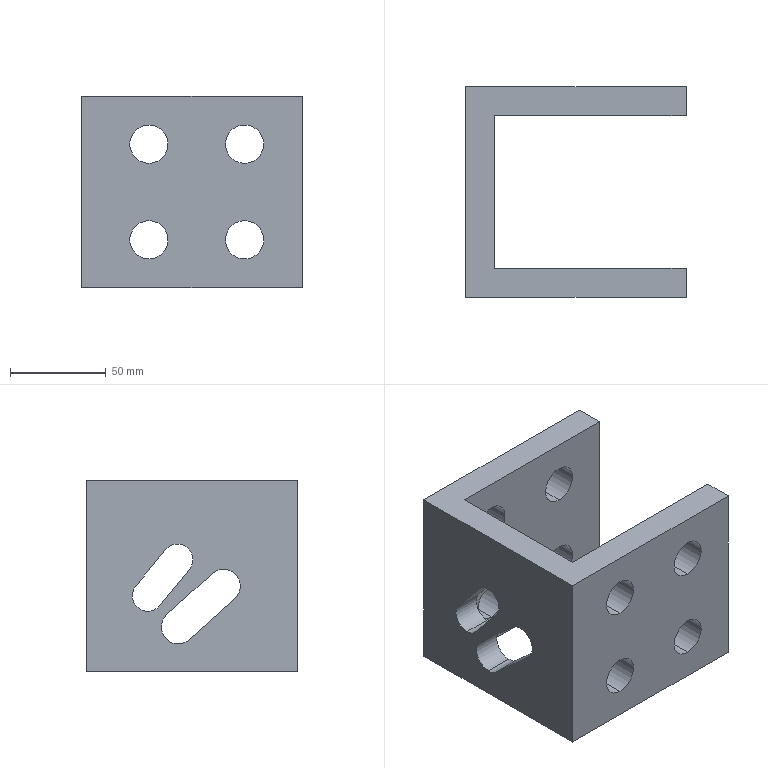Part | SolidWorks | features ICE 2, Extrusion 1 | 1 solid | 36 faces | box 115 x 110 x 100 mm | volume 406186 mm3 | cylinder 22 | plane 14 | commonest cylinder face diameters 20 x16 16.141 x3 17.644 x3
STEP:
#1=CARTESIAN_POINT('',(-15.,47.219,14.48));
#2=VERTEX_POINT('',#1);
#3=CARTESIAN_POINT('',(-15.,53.133,29.848));
#4=VERTEX_POINT('',#3);
#5=CARTESIAN_POINT('',(-15.,47.219,23.302));
#6=DIRECTION('',(1.,0.,0.));
#7=DIRECTION('',(0.,0.,-1.));
#8=AXIS2_PLACEMENT_3D('',#5,#6,#7);
#9=CIRCLE('',#8,8.822);
#10=EDGE_CURVE('',#2,#4,#9,.T.);
#11=ORIENTED_EDGE('',*,*,#10,.F.);
#12=CARTESIAN_POINT('',(0.,47.219,14.48));
#13=VERTEX_POINT('',#12);
#14=CARTESIAN_POINT('',(-500.,47.219,14.48));
#15=DIRECTION('',(1.,0.,0.));
#16=VECTOR('',#15,1000.);
#17=LINE('',#14,#16);
#18=EDGE_CURVE('',#2,#13,#17,.T.);
#19=ORIENTED_EDGE('',*,*,#18,.T.);
#20=CARTESIAN_POINT('',(0.,53.133,29.848));
#21=VERTEX_POINT('',#20);
#22=CARTESIAN_POINT('',(0.,47.219,23.302));
#23=DIRECTION('',(1.,0.,0.));
#24=DIRECTION('',(0.,0.,-1.));
#25=AXIS2_PLACEMENT_3D('',#22,#23,#24);
#26=CIRCLE('',#25,8.822);
#27=EDGE_CURVE('',#13,#21,#26,.T.);
#28=ORIENTED_EDGE('',*,*,#27,.T.);
#29=CARTESIAN_POINT('',(-500.,53.133,29.848));
#30=DIRECTION('',(1.,0.,0.));
#31=VECTOR('',#30,1000.);
#32=LINE('',#29,#31);
#33=EDGE_CURVE('',#4,#21,#32,.T.);
#34=ORIENTED_EDGE('',*,*,#33,.F.);
#35=EDGE_LOOP('',(#11,#19,#28,#34));
#36=FACE_OUTER_BOUND('',#35,.T.);
#37=CARTESIAN_POINT('',(-500.,47.219,23.302));
#38=DIRECTION('',(1.,0.,0.));
#39=DIRECTION('',(0.,0.,-1.));
#40=AXIS2_PLACEMENT_3D('',#37,#38,#39);
#41=CYLINDRICAL_SURFACE('',#40,8.822);
#42=ADVANCED_FACE('',(#36),#41,.F.);
#43=CARTESIAN_POINT('',(-15.,63.133,31.531));
#44=VERTEX_POINT('',#43);
#45=CARTESIAN_POINT('',(-15.,69.375,44.718));
#46=VERTEX_POINT('',#45);
#47=CARTESIAN_POINT('',(-15.,63.133,39.601));
#48=DIRECTION('',(1.,0.,0.));
#49=DIRECTION('',(0.,0.,-1.));
#50=AXIS2_PLACEMENT_3D('',#47,#48,#49);
#51=CIRCLE('',#50,8.071);
#52=EDGE_CURVE('',#44,#46,#51,.T.);
#53=ORIENTED_EDGE('',*,*,#52,.F.);
#54=CARTESIAN_POINT('',(0.,63.133,31.531));
#55=VERTEX_POINT('',#54);
#56=CARTESIAN_POINT('',(-500.,63.133,31.531));
#57=DIRECTION('',(1.,0.,0.));
#58=VECTOR('',#57,1000.);
#59=LINE('',#56,#58);
#60=EDGE_CURVE('',#44,#55,#59,.T.);
#61=ORIENTED_EDGE('',*,*,#60,.T.);
#62=CARTESIAN_POINT('',(0.,69.375,44.718));
#63=VERTEX_POINT('',#62);
#64=CARTESIAN_POINT('',(0.,63.133,39.601));
#65=DIRECTION('',(1.,0.,0.));
#66=DIRECTION('',(0.,0.,-1.));
#67=AXIS2_PLACEMENT_3D('',#64,#65,#66);
#68=CIRCLE('',#67,8.071);
#69=EDGE_CURVE('',#55,#63,#68,.T.);
#70=ORIENTED_EDGE('',*,*,#69,.T.);
#71=CARTESIAN_POINT('',(-500.,69.375,44.718));
#72=DIRECTION('',(1.,0.,0.));
#73=VECTOR('',#72,1000.);
#74=LINE('',#71,#73);
#75=EDGE_CURVE('',#46,#63,#74,.T.);
#76=ORIENTED_EDGE('',*,*,#75,.F.);
#77=EDGE_LOOP('',(#53,#61,#70,#76));
#78=FACE_OUTER_BOUND('',#77,.T.);
#79=CARTESIAN_POINT('',(-500.,63.133,39.601));
#80=DIRECTION('',(1.,0.,0.));
#81=DIRECTION('',(0.,0.,-1.));
#82=AXIS2_PLACEMENT_3D('',#79,#80,#81);
#83=CYLINDRICAL_SURFACE('',#82,8.071);
#84=ADVANCED_FACE('',(#78),#83,.F.);
#85=CARTESIAN_POINT('',(70.,80.,15.));
#86=VERTEX_POINT('',#85);
#87=CARTESIAN_POINT('',(70.,80.,35.));
#88=VERTEX_POINT('',#87);
#89=CARTESIAN_POINT('',(70.,80.,25.));
#90=DIRECTION('',(0.,1.,0.));
#91=DIRECTION('',(0.,0.,1.));
#92=AXIS2_PLACEMENT_3D('',#89,#90,#91);
#93=CIRCLE('',#92,10.);
#94=EDGE_CURVE('',#86,#88,#93,.T.);
#95=ORIENTED_EDGE('',*,*,#94,.F.);
#96=CARTESIAN_POINT('',(70.,95.,15.));
#97=VERTEX_POINT('',#96);
#98=CARTESIAN_POINT('',(70.,-405.,15.));
#99=DIRECTION('',(0.,1.,0.));
#100=VECTOR('',#99,1000.);
#101=LINE('',#98,#100);
#102=EDGE_CURVE('',#86,#97,#101,.T.);
#103=ORIENTED_EDGE('',*,*,#102,.T.);
#104=CARTESIAN_POINT('',(70.,95.,35.));
#105=VERTEX_POINT('',#104);
#106=CARTESIAN_POINT('',(70.,95.,25.));
#107=DIRECTION('',(0.,1.,0.));
#108=DIRECTION('',(0.,0.,1.));
#109=AXIS2_PLACEMENT_3D('',#106,#107,#108);
#110=CIRCLE('',#109,10.);
#111=EDGE_CURVE('',#97,#105,#110,.T.);
#112=ORIENTED_EDGE('',*,*,#111,.T.);
#113=CARTESIAN_POINT('',(70.,-405.,35.));
#114=DIRECTION('',(0.,1.,0.));
#115=VECTOR('',#114,1000.);
#116=LINE('',#113,#115);
#117=EDGE_CURVE('',#88,#105,#116,.T.);
#118=ORIENTED_EDGE('',*,*,#117,.F.);
#119=EDGE_LOOP('',(#95,#103,#112,#118));
#120=FACE_OUTER_BOUND('',#119,.T.);
#121=CARTESIAN_POINT('',(70.,-405.,25.));
#122=DIRECTION('',(0.,1.,0.));
#123=DIRECTION('',(0.,0.,1.));
#124=AXIS2_PLACEMENT_3D('',#121,#122,#123);
#125=CYLINDRICAL_SURFACE('',#124,10.);
#126=ADVANCED_FACE('',(#120),#125,.F.);
#127=CARTESIAN_POINT('',(20.,80.,65.));
#128=VERTEX_POINT('',#127);
#129=CARTESIAN_POINT('',(20.,80.,85.));
#130=VERTEX_POINT('',#129);
#131=CARTESIAN_POINT('',(20.,80.,75.));
#132=DIRECTION('',(0.,1.,0.));
#133=DIRECTION('',(0.,0.,1.));
#134=AXIS2_PLACEMENT_3D('',#131,#132,#133);
#135=CIRCLE('',#134,10.);
#136=EDGE_CURVE('',#128,#130,#135,.T.);
#137=ORIENTED_EDGE('',*,*,#136,.F.);
#138=CARTESIAN_POINT('',(20.,95.,65.));
#139=VERTEX_POINT('',#138);
#140=CARTESIAN_POINT('',(20.,-405.,65.));
#141=DIRECTION('',(0.,1.,0.));
#142=VECTOR('',#141,1000.);
#143=LINE('',#140,#142);
#144=EDGE_CURVE('',#128,#139,#143,.T.);
#145=ORIENTED_EDGE('',*,*,#144,.T.);
#146=CARTESIAN_POINT('',(20.,95.,85.));
#147=VERTEX_POINT('',#146);
#148=CARTESIAN_POINT('',(20.,95.,75.));
#149=DIRECTION('',(0.,1.,0.));
#150=DIRECTION('',(0.,0.,1.));
#151=AXIS2_PLACEMENT_3D('',#148,#149,#150);
#152=CIRCLE('',#151,10.);
#153=EDGE_CURVE('',#139,#147,#152,.T.);
#154=ORIENTED_EDGE('',*,*,#153,.T.);
#155=CARTESIAN_POINT('',(20.,-405.,85.));
#156=DIRECTION('',(0.,1.,0.));
#157=VECTOR('',#156,1000.);
#158=LINE('',#155,#157);
#159=EDGE_CURVE('',#130,#147,#158,.T.);
#160=ORIENTED_EDGE('',*,*,#159,.F.);
#161=EDGE_LOOP('',(#137,#145,#154,#160));
#162=FACE_OUTER_BOUND('',#161,.T.);
#163=CARTESIAN_POINT('',(20.,-405.,75.));
#164=DIRECTION('',(0.,1.,0.));
#165=DIRECTION('',(0.,0.,1.));
#166=AXIS2_PLACEMENT_3D('',#163,#164,#165);
#167=CYLINDRICAL_SURFACE('',#166,10.);
#168=ADVANCED_FACE('',(#162),#167,.F.);
#169=CARTESIAN_POINT('',(70.,80.,65.));
#170=VERTEX_POINT('',#169);
#171=CARTESIAN_POINT('',(70.,80.,85.));
#172=VERTEX_POINT('',#171);
#173=CARTESIAN_POINT('',(70.,80.,75.));
#174=DIRECTION('',(0.,1.,0.));
#175=DIRECTION('',(0.,0.,1.));
#176=AXIS2_PLACEMENT_3D('',#173,#174,#175);
#177=CIRCLE('',#176,10.);
#178=EDGE_CURVE('',#170,#172,#177,.T.);
#179=ORIENTED_EDGE('',*,*,#178,.F.);
#180=CARTESIAN_POINT('',(70.,95.,65.));
#181=VERTEX_POINT('',#180);
#182=CARTESIAN_POINT('',(70.,-405.,65.));
#183=DIRECTION('',(0.,1.,0.));
#184=VECTOR('',#183,1000.);
#185=LINE('',#182,#184);
#186=EDGE_CURVE('',#170,#181,#185,.T.);
#187=ORIENTED_EDGE('',*,*,#186,.T.);
#188=CARTESIAN_POINT('',(70.,95.,85.));
#189=VERTEX_POINT('',#188);
#190=CARTESIAN_POINT('',(70.,95.,75.));
#191=DIRECTION('',(0.,1.,0.));
#192=DIRECTION('',(0.,0.,1.));
#193=AXIS2_PLACEMENT_3D('',#190,#191,#192);
#194=CIRCLE('',#193,10.);
#195=EDGE_CURVE('',#181,#189,#194,.T.);
#196=ORIENTED_EDGE('',*,*,#195,.T.);
#197=CARTESIAN_POINT('',(70.,-405.,85.));
#198=DIRECTION('',(0.,1.,0.));
#199=VECTOR('',#198,1000.);
#200=LINE('',#197,#199);
#201=EDGE_CURVE('',#172,#189,#200,.T.);
#202=ORIENTED_EDGE('',*,*,#201,.F.);
#203=EDGE_LOOP('',(#179,#187,#196,#202));
#204=FACE_OUTER_BOUND('',#203,.T.);
#205=CARTESIAN_POINT('',(70.,-405.,75.));
#206=DIRECTION('',(0.,1.,0.));
#207=DIRECTION('',(0.,0.,1.));
#208=AXIS2_PLACEMENT_3D('',#205,#206,#207);
#209=CYLINDRICAL_SURFACE('',#208,10.);
#210=ADVANCED_FACE('',(#204),#209,.F.);
#211=CARTESIAN_POINT('',(20.,80.,15.));
#212=VERTEX_POINT('',#211);
#213=CARTESIAN_POINT('',(20.,80.,35.));
#214=VERTEX_POINT('',#213);
#215=CARTESIAN_POINT('',(20.,80.,25.));
#216=DIRECTION('',(0.,1.,0.));
#217=DIRECTION('',(0.,0.,1.));
#218=AXIS2_PLACEMENT_3D('',#215,#216,#217);
#219=CIRCLE('',#218,10.);
#220=EDGE_CURVE('',#212,#214,#219,.T.);
#221=ORIENTED_EDGE('',*,*,#220,.F.);
#222=CARTESIAN_POINT('',(20.,95.,15.));
#223=VERTEX_POINT('',#222);
#224=CARTESIAN_POINT('',(20.,-405.,15.));
#225=DIRECTION('',(0.,1.,0.));
#226=VECTOR('',#225,1000.);
#227=LINE('',#224,#226);
#228=EDGE_CURVE('',#212,#223,#227,.T.);
#229=ORIENTED_EDGE('',*,*,#228,.T.);
#230=CARTESIAN_POINT('',(20.,95.,35.));
#231=VERTEX_POINT('',#230);
#232=CARTESIAN_POINT('',(20.,95.,25.));
#233=DIRECTION('',(0.,1.,0.));
#234=DIRECTION('',(0.,0.,1.));
#235=AXIS2_PLACEMENT_3D('',#232,#233,#234);
#236=CIRCLE('',#235,10.);
#237=EDGE_CURVE('',#223,#231,#236,.T.);
#238=ORIENTED_EDGE('',*,*,#237,.T.);
#239=CARTESIAN_POINT('',(20.,-405.,35.));
#240=DIRECTION('',(0.,1.,0.));
#241=VECTOR('',#240,1000.);
#242=LINE('',#239,#241);
#243=EDGE_CURVE('',#214,#231,#242,.T.);
#244=ORIENTED_EDGE('',*,*,#243,.F.);
#245=EDGE_LOOP('',(#221,#229,#238,#244));
#246=FACE_OUTER_BOUND('',#245,.T.);
#247=CARTESIAN_POINT('',(20.,-405.,25.));
#248=DIRECTION('',(0.,1.,0.));
#249=DIRECTION('',(0.,0.,1.));
#250=AXIS2_PLACEMENT_3D('',#247,#248,#249);
#251=CYLINDRICAL_SURFACE('',#250,10.);
#252=ADVANCED_FACE('',(#246),#251,.F.);
#253=CARTESIAN_POINT('',(70.,-15.,15.));
#254=VERTEX_POINT('',#253);
#255=CARTESIAN_POINT('',(70.,-15.,35.));
#256=VERTEX_POINT('',#255);
#257=CARTESIAN_POINT('',(70.,-15.,25.));
#258=DIRECTION('',(0.,1.,0.));
#259=DIRECTION('',(0.,0.,1.));
#260=AXIS2_PLACEMENT_3D('',#257,#258,#259);
#261=CIRCLE('',#260,10.);
#262=EDGE_CURVE('',#254,#256,#261,.T.);
#263=ORIENTED_EDGE('',*,*,#262,.F.);
#264=CARTESIAN_POINT('',(70.,0.,15.));
#265=VERTEX_POINT('',#264);
#266=CARTESIAN_POINT('',(70.,-405.,15.));
#267=DIRECTION('',(0.,1.,0.));
#268=VECTOR('',#267,1000.);
#269=LINE('',#266,#268);
#270=EDGE_CURVE('',#254,#265,#269,.T.);
#271=ORIENTED_EDGE('',*,*,#270,.T.);
#272=CARTESIAN_POINT('',(70.,0.,35.));
#273=VERTEX_POINT('',#272);
#274=CARTESIAN_POINT('',(70.,0.,25.));
#275=DIRECTION('',(0.,-1.,0.));
#276=DIRECTION('',(0.,0.,-1.));
#277=AXIS2_PLACEMENT_3D('',#274,#275,#276);
#278=CIRCLE('',#277,10.);
#279=EDGE_CURVE('',#273,#265,#278,.T.);
#280=ORIENTED_EDGE('',*,*,#279,.F.);
#281=CARTESIAN_POINT('',(70.,-405.,35.));
#282=DIRECTION('',(0.,1.,0.));
#283=VECTOR('',#282,1000.);
#284=LINE('',#281,#283);
#285=EDGE_CURVE('',#256,#273,#284,.T.);
#286=ORIENTED_EDGE('',*,*,#285,.F.);
#287=EDGE_LOOP('',(#263,#271,#280,#286));
#288=FACE_OUTER_BOUND('',#287,.T.);
#289=CARTESIAN_POINT('',(70.,-405.,25.));
#290=DIRECTION('',(0.,1.,0.));
#291=DIRECTION('',(0.,0.,1.));
#292=AXIS2_PLACEMENT_3D('',#289,#290,#291);
#293=CYLINDRICAL_SURFACE('',#292,10.);
#294=ADVANCED_FACE('',(#288),#293,.F.);
#295=CARTESIAN_POINT('',(20.,-15.,65.));
#296=VERTEX_POINT('',#295);
#297=CARTESIAN_POINT('',(20.,-15.,85.));
#298=VERTEX_POINT('',#297);
#299=CARTESIAN_POINT('',(20.,-15.,75.));
#300=DIRECTION('',(0.,1.,0.));
#301=DIRECTION('',(0.,0.,1.));
#302=AXIS2_PLACEMENT_3D('',#299,#300,#301);
#303=CIRCLE('',#302,10.);
#304=EDGE_CURVE('',#296,#298,#303,.T.);
#305=ORIENTED_EDGE('',*,*,#304,.F.);
#306=CARTESIAN_POINT('',(20.,0.,65.));
#307=VERTEX_POINT('',#306);
#308=CARTESIAN_POINT('',(20.,-405.,65.));
#309=DIRECTION('',(0.,1.,0.));
#310=VECTOR('',#309,1000.);
#311=LINE('',#308,#310);
#312=EDGE_CURVE('',#296,#307,#311,.T.);
#313=ORIENTED_EDGE('',*,*,#312,.T.);
#314=CARTESIAN_POINT('',(20.,0.,85.));
#315=VERTEX_POINT('',#314);
#316=CARTESIAN_POINT('',(20.,0.,75.));
#317=DIRECTION('',(0.,-1.,0.));
#318=DIRECTION('',(0.,0.,-1.));
#319=AXIS2_PLACEMENT_3D('',#316,#317,#318);
#320=CIRCLE('',#319,10.);
#321=EDGE_CURVE('',#315,#307,#320,.T.);
#322=ORIENTED_EDGE('',*,*,#321,.F.);
#323=CARTESIAN_POINT('',(20.,-405.,85.));
#324=DIRECTION('',(0.,1.,0.));
#325=VECTOR('',#324,1000.);
#326=LINE('',#323,#325);
#327=EDGE_CURVE('',#298,#315,#326,.T.);
#328=ORIENTED_EDGE('',*,*,#327,.F.);
#329=EDGE_LOOP('',(#305,#313,#322,#328));
#330=FACE_OUTER_BOUND('',#329,.T.);
#331=CARTESIAN_POINT('',(20.,-405.,75.));
#332=DIRECTION('',(0.,1.,0.));
#333=DIRECTION('',(0.,0.,1.));
#334=AXIS2_PLACEMENT_3D('',#331,#332,#333);
#335=CYLINDRICAL_SURFACE('',#334,10.);
#336=ADVANCED_FACE('',(#330),#335,.F.);
#337=CARTESIAN_POINT('',(70.,-15.,65.));
#338=VERTEX_POINT('',#337);
#339=CARTESIAN_POINT('',(70.,-15.,85.));
#340=VERTEX_POINT('',#339);
#341=CARTESIAN_POINT('',(70.,-15.,75.));
#342=DIRECTION('',(0.,1.,0.));
#343=DIRECTION('',(0.,0.,1.));
#344=AXIS2_PLACEMENT_3D('',#341,#342,#343);
#345=CIRCLE('',#344,10.);
#346=EDGE_CURVE('',#338,#340,#345,.T.);
#347=ORIENTED_EDGE('',*,*,#346,.F.);
#348=CARTESIAN_POINT('',(70.,0.,65.));
#349=VERTEX_POINT('',#348);
#350=CARTESIAN_POINT('',(70.,-405.,65.));
#351=DIRECTION('',(0.,1.,0.));
#352=VECTOR('',#351,1000.);
#353=LINE('',#350,#352);
#354=EDGE_CURVE('',#338,#349,#353,.T.);
#355=ORIENTED_EDGE('',*,*,#354,.T.);
#356=CARTESIAN_POINT('',(70.,0.,85.));
#357=VERTEX_POINT('',#356);
#358=CARTESIAN_POINT('',(70.,0.,75.));
#359=DIRECTION('',(0.,-1.,0.));
#360=DIRECTION('',(0.,0.,-1.));
#361=AXIS2_PLACEMENT_3D('',#358,#359,#360);
#362=CIRCLE('',#361,10.);
#363=EDGE_CURVE('',#357,#349,#362,.T.);
#364=ORIENTED_EDGE('',*,*,#363,.F.);
#365=CARTESIAN_POINT('',(70.,-405.,85.));
#366=DIRECTION('',(0.,1.,0.));
#367=VECTOR('',#366,1000.);
#368=LINE('',#365,#367);
#369=EDGE_CURVE('',#340,#357,#368,.T.);
#370=ORIENTED_EDGE('',*,*,#369,.F.);
#371=EDGE_LOOP('',(#347,#355,#364,#370));
#372=FACE_OUTER_BOUND('',#371,.T.);
#373=CARTESIAN_POINT('',(70.,-405.,75.));
#374=DIRECTION('',(0.,1.,0.));
#375=DIRECTION('',(0.,0.,1.));
#376=AXIS2_PLACEMENT_3D('',#373,#374,#375);
#377=CYLINDRICAL_SURFACE('',#376,10.);
#378=ADVANCED_FACE('',(#372),#377,.F.);
#379=CARTESIAN_POINT('',(20.,-15.,15.));
#380=VERTEX_POINT('',#379);
#381=CARTESIAN_POINT('',(20.,-15.,35.));
#382=VERTEX_POINT('',#381);
#383=CARTESIAN_POINT('',(20.,-15.,25.));
#384=DIRECTION('',(0.,1.,0.));
#385=DIRECTION('',(0.,0.,1.));
#386=AXIS2_PLACEMENT_3D('',#383,#384,#385);
#387=CIRCLE('',#386,10.);
#388=EDGE_CURVE('',#380,#382,#387,.T.);
#389=ORIENTED_EDGE('',*,*,#388,.F.);
#390=CARTESIAN_POINT('',(20.,0.,15.));
#391=VERTEX_POINT('',#390);
#392=CARTESIAN_POINT('',(20.,-405.,15.));
#393=DIRECTION('',(0.,1.,0.));
#394=VECTOR('',#393,1000.);
#395=LINE('',#392,#394);
#396=EDGE_CURVE('',#380,#391,#395,.T.);
#397=ORIENTED_EDGE('',*,*,#396,.T.);
#398=CARTESIAN_POINT('',(20.,0.,35.));
#399=VERTEX_POINT('',#398);
#400=CARTESIAN_POINT('',(20.,0.,25.));
#401=DIRECTION('',(0.,-1.,0.));
#402=DIRECTION('',(0.,0.,-1.));
#403=AXIS2_PLACEMENT_3D('',#400,#401,#402);
#404=CIRCLE('',#403,10.);
#405=EDGE_CURVE('',#399,#391,#404,.T.);
#406=ORIENTED_EDGE('',*,*,#405,.F.);
#407=CARTESIAN_POINT('',(20.,-405.,35.));
#408=DIRECTION('',(0.,1.,0.));
#409=VECTOR('',#408,1000.);
#410=LINE('',#407,#409);
#411=EDGE_CURVE('',#382,#399,#410,.T.);
#412=ORIENTED_EDGE('',*,*,#411,.F.);
#413=EDGE_LOOP('',(#389,#397,#406,#412));
#414=FACE_OUTER_BOUND('',#413,.T.);
#415=CARTESIAN_POINT('',(20.,-405.,25.));
#416=DIRECTION('',(0.,1.,0.));
#417=DIRECTION('',(0.,0.,1.));
#418=AXIS2_PLACEMENT_3D('',#415,#416,#417);
#419=CYLINDRICAL_SURFACE('',#418,10.);
#420=ADVANCED_FACE('',(#414),#419,.F.);
#421=CARTESIAN_POINT('',(0.,17.684,38.097));
#422=VERTEX_POINT('',#421);
#423=CARTESIAN_POINT('',(0.,41.305,16.756));
#424=VERTEX_POINT('',#423);
#425=CARTESIAN_POINT('',(0.,17.684,38.097));
#426=DIRECTION('',(0.,0.742,-0.6704));
#427=VECTOR('',#426,1000.);
#428=LINE('',#425,#427);
#429=EDGE_CURVE('',#422,#424,#428,.T.);
#430=ORIENTED_EDGE('',*,*,#429,.F.);
#431=CARTESIAN_POINT('',(0.,29.512,51.189));
#432=VERTEX_POINT('',#431);
#433=CARTESIAN_POINT('',(0.,23.598,44.643));
#434=DIRECTION('',(1.,0.,0.));
#435=DIRECTION('',(0.,0.,-1.));
#436=AXIS2_PLACEMENT_3D('',#433,#434,#435);
#437=CIRCLE('',#436,8.822);
#438=EDGE_CURVE('',#432,#422,#437,.T.);
#439=ORIENTED_EDGE('',*,*,#438,.F.);
#440=CARTESIAN_POINT('',(0.,29.512,51.189));
#441=DIRECTION('',(0.,-0.742,0.6704));
#442=VECTOR('',#441,1000.);
#443=LINE('',#440,#442);
#444=EDGE_CURVE('',#21,#432,#443,.T.);
#445=ORIENTED_EDGE('',*,*,#444,.F.);
#446=ORIENTED_EDGE('',*,*,#27,.F.);
#447=CARTESIAN_POINT('',(0.,47.219,23.302));
#448=DIRECTION('',(1.,0.,0.));
#449=DIRECTION('',(0.,0.,-1.));
#450=AXIS2_PLACEMENT_3D('',#447,#448,#449);
#451=CIRCLE('',#450,8.822);
#452=EDGE_CURVE('',#424,#13,#451,.T.);
#453=ORIENTED_EDGE('',*,*,#452,.F.);
#454=EDGE_LOOP('',(#430,#439,#445,#446,#453));
#455=FACE_BOUND('',#454,.T.);
#456=CARTESIAN_POINT('',(0.,41.305,53.501));
#457=VERTEX_POINT('',#456);
#458=CARTESIAN_POINT('',(0.,56.891,34.485));
#459=VERTEX_POINT('',#458);
#460=CARTESIAN_POINT('',(0.,41.305,53.501));
#461=DIRECTION('',(0.,0.6339,-0.7734));
#462=VECTOR('',#461,1000.);
#463=LINE('',#460,#462);
#464=EDGE_CURVE('',#457,#459,#463,.T.);
#465=ORIENTED_EDGE('',*,*,#464,.F.);
#466=CARTESIAN_POINT('',(0.,53.788,63.733));
#467=VERTEX_POINT('',#466);
#468=CARTESIAN_POINT('',(0.,47.547,58.617));
#469=DIRECTION('',(1.,0.,0.));
#470=DIRECTION('',(0.,0.,-1.));
#471=AXIS2_PLACEMENT_3D('',#468,#469,#470);
#472=CIRCLE('',#471,8.071);
#473=EDGE_CURVE('',#467,#457,#472,.T.);
#474=ORIENTED_EDGE('',*,*,#473,.F.);
#475=CARTESIAN_POINT('',(0.,53.788,63.733));
#476=DIRECTION('',(0.,-0.6339,0.7734));
#477=VECTOR('',#476,1000.);
#478=LINE('',#475,#477);
#479=EDGE_CURVE('',#63,#467,#478,.T.);
#480=ORIENTED_EDGE('',*,*,#479,.F.);
#481=ORIENTED_EDGE('',*,*,#69,.F.);
#482=CARTESIAN_POINT('',(0.,63.133,39.601));
#483=DIRECTION('',(1.,0.,0.));
#484=DIRECTION('',(0.,0.,-1.));
#485=AXIS2_PLACEMENT_3D('',#482,#483,#484);
#486=CIRCLE('',#485,8.071);
#487=EDGE_CURVE('',#459,#55,#486,.T.);
#488=ORIENTED_EDGE('',*,*,#487,.F.);
#489=EDGE_LOOP('',(#465,#474,#480,#481,#488));
#490=FACE_BOUND('',#489,.T.);
#491=CARTESIAN_POINT('',(0.,0.,0.));
#492=VERTEX_POINT('',#491);
#493=CARTESIAN_POINT('',(0.,80.,0.));
#494=VERTEX_POINT('',#493);
#495=CARTESIAN_POINT('',(0.,0.,0.));
#496=DIRECTION('',(0.,1.,0.));
#497=VECTOR('',#496,1000.);
#498=LINE('',#495,#497);
#499=EDGE_CURVE('',#492,#494,#498,.T.);
#500=ORIENTED_EDGE('',*,*,#499,.T.);
#501=CARTESIAN_POINT('',(0.,80.,100.));
#502=VERTEX_POINT('',#501);
#503=CARTESIAN_POINT('',(0.,80.,100.));
#504=DIRECTION('',(0.,0.,-1.));
#505=VECTOR('',#504,1000.);
#506=LINE('',#503,#505);
#507=EDGE_CURVE('',#502,#494,#506,.T.);
#508=ORIENTED_EDGE('',*,*,#507,.F.);
#509=CARTESIAN_POINT('',(0.,0.,100.));
#510=VERTEX_POINT('',#509);
#511=CARTESIAN_POINT('',(0.,0.,100.));
#512=DIRECTION('',(0.,1.,0.));
#513=VECTOR('',#512,1000.);
#514=LINE('',#511,#513);
#515=EDGE_CURVE('',#510,#502,#514,.T.);
#516=ORIENTED_EDGE('',*,*,#515,.F.);
#517=CARTESIAN_POINT('',(0.,0.,100.));
#518=DIRECTION('',(0.,0.,-1.));
#519=VECTOR('',#518,1000.);
#520=LINE('',#517,#519);
#521=EDGE_CURVE('',#510,#492,#520,.T.);
#522=ORIENTED_EDGE('',*,*,#521,.T.);
#523=EDGE_LOOP('',(#500,#508,#516,#522));
#524=FACE_OUTER_BOUND('',#523,.T.);
#525=CARTESIAN_POINT('',(0.,0.,100.));
#526=DIRECTION('',(-1.,0.,0.));
#527=DIRECTION('',(0.,0.,1.));
#528=AXIS2_PLACEMENT_3D('',#525,#526,#527);
#529=PLANE('',#528);
#530=ADVANCED_FACE('',(#455,#490,#524),#529,.F.);
#531=CARTESIAN_POINT('',(70.,80.,25.));
#532=DIRECTION('',(0.,1.,0.));
#533=DIRECTION('',(0.,0.,1.));
#534=AXIS2_PLACEMENT_3D('',#531,#532,#533);
#535=CIRCLE('',#534,10.);
#536=EDGE_CURVE('',#88,#86,#535,.T.);
#537=ORIENTED_EDGE('',*,*,#536,.T.);
#538=ORIENTED_EDGE('',*,*,#94,.T.);
#539=EDGE_LOOP('',(#537,#538));
#540=FACE_BOUND('',#539,.T.);
#541=CARTESIAN_POINT('',(20.,80.,75.));
#542=DIRECTION('',(0.,1.,0.));
#543=DIRECTION('',(0.,0.,1.));
#544=AXIS2_PLACEMENT_3D('',#541,#542,#543);
#545=CIRCLE('',#544,10.);
#546=EDGE_CURVE('',#130,#128,#545,.T.);
#547=ORIENTED_EDGE('',*,*,#546,.T.);
#548=ORIENTED_EDGE('',*,*,#136,.T.);
#549=EDGE_LOOP('',(#547,#548));
#550=FACE_BOUND('',#549,.T.);
#551=CARTESIAN_POINT('',(70.,80.,75.));
#552=DIRECTION('',(0.,1.,0.));
#553=DIRECTION('',(0.,0.,1.));
#554=AXIS2_PLACEMENT_3D('',#551,#552,#553);
#555=CIRCLE('',#554,10.);
#556=EDGE_CURVE('',#172,#170,#555,.T.);
#557=ORIENTED_EDGE('',*,*,#556,.T.);
#558=ORIENTED_EDGE('',*,*,#178,.T.);
#559=EDGE_LOOP('',(#557,#558));
#560=FACE_BOUND('',#559,.T.);
#561=CARTESIAN_POINT('',(20.,80.,25.));
#562=DIRECTION('',(0.,1.,0.));
#563=DIRECTION('',(0.,0.,1.));
#564=AXIS2_PLACEMENT_3D('',#561,#562,#563);
#565=CIRCLE('',#564,10.);
#566=EDGE_CURVE('',#214,#212,#565,.T.);
#567=ORIENTED_EDGE('',*,*,#566,.T.);
#568=ORIENTED_EDGE('',*,*,#220,.T.);
#569=EDGE_LOOP('',(#567,#568));
#570=FACE_BOUND('',#569,.T.);
#571=CARTESIAN_POINT('',(100.,80.,0.));
#572=VERTEX_POINT('',#571);
#573=CARTESIAN_POINT('',(0.,80.,0.));
#574=DIRECTION('',(1.,0.,0.));
#575=VECTOR('',#574,1000.);
#576=LINE('',#573,#575);
#577=EDGE_CURVE('',#494,#572,#576,.T.);
#578=ORIENTED_EDGE('',*,*,#577,.T.);
#579=CARTESIAN_POINT('',(100.,80.,100.));
#580=VERTEX_POINT('',#579);
#581=CARTESIAN_POINT('',(100.,80.,100.));
#582=DIRECTION('',(0.,0.,-1.));
#583=VECTOR('',#582,1000.);
#584=LINE('',#581,#583);
#585=EDGE_CURVE('',#580,#572,#584,.T.);
#586=ORIENTED_EDGE('',*,*,#585,.F.);
#587=CARTESIAN_POINT('',(0.,80.,100.));
#588=DIRECTION('',(1.,0.,0.));
#589=VECTOR('',#588,1000.);
#590=LINE('',#587,#589);
#591=EDGE_CURVE('',#502,#580,#590,.T.);
#592=ORIENTED_EDGE('',*,*,#591,.F.);
#593=ORIENTED_EDGE('',*,*,#507,.T.);
#594=EDGE_LOOP('',(#578,#586,#592,#593));
#595=FACE_OUTER_BOUND('',#594,.T.);
#596=CARTESIAN_POINT('',(0.,80.,100.));
#597=DIRECTION('',(0.,1.,0.));
#598=DIRECTION('',(0.,0.,1.));
#599=AXIS2_PLACEMENT_3D('',#596,#597,#598);
#600=PLANE('',#599);
#601=ADVANCED_FACE('',(#540,#550,#560,#570,#595),#600,.F.);
#602=CARTESIAN_POINT('',(100.,95.,0.));
#603=VERTEX_POINT('',#602);
#604=CARTESIAN_POINT('',(100.,95.,0.));
#605=DIRECTION('',(0.,1.,0.));
#606=VECTOR('',#605,1000.);
#607=LINE('',#604,#606);
#608=EDGE_CURVE('',#572,#603,#607,.T.);
#609=ORIENTED_EDGE('',*,*,#608,.T.);
#610=CARTESIAN_POINT('',(100.,95.,100.));
#611=VERTEX_POINT('',#610);
#612=CARTESIAN_POINT('',(100.,95.,100.));
#613=DIRECTION('',(0.,0.,-1.));
#614=VECTOR('',#613,1000.);
#615=LINE('',#612,#614);
#616=EDGE_CURVE('',#611,#603,#615,.T.);
#617=ORIENTED_EDGE('',*,*,#616,.F.);
#618=CARTESIAN_POINT('',(100.,95.,100.));
#619=DIRECTION('',(0.,1.,0.));
#620=VECTOR('',#619,1000.);
#621=LINE('',#618,#620);
#622=EDGE_CURVE('',#580,#611,#621,.T.);
#623=ORIENTED_EDGE('',*,*,#622,.F.);
#624=ORIENTED_EDGE('',*,*,#585,.T.);
#625=EDGE_LOOP('',(#609,#617,#623,#624));
#626=FACE_OUTER_BOUND('',#625,.T.);
#627=CARTESIAN_POINT('',(100.,95.,100.));
#628=DIRECTION('',(-1.,0.,0.));
#629=DIRECTION('',(0.,0.,1.));
#630=AXIS2_PLACEMENT_3D('',#627,#628,#629);
#631=PLANE('',#630);
#632=ADVANCED_FACE('',(#626),#631,.F.);
#633=CARTESIAN_POINT('',(70.,95.,25.));
#634=DIRECTION('',(0.,1.,0.));
#635=DIRECTION('',(0.,0.,1.));
#636=AXIS2_PLACEMENT_3D('',#633,#634,#635);
#637=CIRCLE('',#636,10.);
#638=EDGE_CURVE('',#105,#97,#637,.T.);
#639=ORIENTED_EDGE('',*,*,#638,.F.);
#640=ORIENTED_EDGE('',*,*,#111,.F.);
#641=EDGE_LOOP('',(#639,#640));
#642=FACE_BOUND('',#641,.T.);
#643=CARTESIAN_POINT('',(20.,95.,75.));
#644=DIRECTION('',(0.,1.,0.));
#645=DIRECTION('',(0.,0.,1.));
#646=AXIS2_PLACEMENT_3D('',#643,#644,#645);
#647=CIRCLE('',#646,10.);
#648=EDGE_CURVE('',#147,#139,#647,.T.);
#649=ORIENTED_EDGE('',*,*,#648,.F.);
#650=ORIENTED_EDGE('',*,*,#153,.F.);
#651=EDGE_LOOP('',(#649,#650));
#652=FACE_BOUND('',#651,.T.);
#653=CARTESIAN_POINT('',(70.,95.,75.));
#654=DIRECTION('',(0.,1.,0.));
#655=DIRECTION('',(0.,0.,1.));
#656=AXIS2_PLACEMENT_3D('',#653,#654,#655);
#657=CIRCLE('',#656,10.);
#658=EDGE_CURVE('',#189,#181,#657,.T.);
#659=ORIENTED_EDGE('',*,*,#658,.F.);
#660=ORIENTED_EDGE('',*,*,#195,.F.);
#661=EDGE_LOOP('',(#659,#660));
#662=FACE_BOUND('',#661,.T.);
#663=CARTESIAN_POINT('',(20.,95.,25.));
#664=DIRECTION('',(0.,1.,0.));
#665=DIRECTION('',(0.,0.,1.));
#666=AXIS2_PLACEMENT_3D('',#663,#664,#665);
#667=CIRCLE('',#666,10.);
#668=EDGE_CURVE('',#231,#223,#667,.T.);
#669=ORIENTED_EDGE('',*,*,#668,.F.);
#670=ORIENTED_EDGE('',*,*,#237,.F.);
#671=EDGE_LOOP('',(#669,#670));
#672=FACE_BOUND('',#671,.T.);
#673=CARTESIAN_POINT('',(-15.,95.,0.));
#674=VERTEX_POINT('',#673);
#675=CARTESIAN_POINT('',(-15.,95.,0.));
#676=DIRECTION('',(-1.,0.,0.));
#677=VECTOR('',#676,1000.);
#678=LINE('',#675,#677);
#679=EDGE_CURVE('',#603,#674,#678,.T.);
#680=ORIENTED_EDGE('',*,*,#679,.T.);
#681=CARTESIAN_POINT('',(-15.,95.,100.));
#682=VERTEX_POINT('',#681);
#683=CARTESIAN_POINT('',(-15.,95.,100.));
#684=DIRECTION('',(0.,0.,-1.));
#685=VECTOR('',#684,1000.);
#686=LINE('',#683,#685);
#687=EDGE_CURVE('',#682,#674,#686,.T.);
#688=ORIENTED_EDGE('',*,*,#687,.F.);
#689=CARTESIAN_POINT('',(-15.,95.,100.));
#690=DIRECTION('',(-1.,0.,0.));
#691=VECTOR('',#690,1000.);
#692=LINE('',#689,#691);
#693=EDGE_CURVE('',#611,#682,#692,.T.);
#694=ORIENTED_EDGE('',*,*,#693,.F.);
#695=ORIENTED_EDGE('',*,*,#616,.T.);
#696=EDGE_LOOP('',(#680,#688,#694,#695));
#697=FACE_OUTER_BOUND('',#696,.T.);
#698=CARTESIAN_POINT('',(-15.,95.,100.));
#699=DIRECTION('',(0.,-1.,0.));
#700=DIRECTION('',(0.,0.,-1.));
#701=AXIS2_PLACEMENT_3D('',#698,#699,#700);
#702=PLANE('',#701);
#703=ADVANCED_FACE('',(#642,#652,#662,#672,#697),#702,.F.);
#704=CARTESIAN_POINT('',(-15.,29.512,51.189));
#705=VERTEX_POINT('',#704);
#706=CARTESIAN_POINT('',(-15.,-19.275,95.268));
#707=DIRECTION('',(0.,-0.742,0.6704));
#708=VECTOR('',#707,1000.);
#709=LINE('',#706,#708);
#710=EDGE_CURVE('',#4,#705,#709,.T.);
#711=ORIENTED_EDGE('',*,*,#710,.T.);
#712=CARTESIAN_POINT('',(-15.,17.684,38.097));
#713=VERTEX_POINT('',#712);
#714=CARTESIAN_POINT('',(-15.,23.598,44.643));
#715=DIRECTION('',(1.,0.,0.));
#716=DIRECTION('',(0.,0.,-1.));
#717=AXIS2_PLACEMENT_3D('',#714,#715,#716);
#718=CIRCLE('',#717,8.822);
#719=EDGE_CURVE('',#705,#713,#718,.T.);
#720=ORIENTED_EDGE('',*,*,#719,.T.);
#721=CARTESIAN_POINT('',(-15.,41.305,16.756));
#722=VERTEX_POINT('',#721);
#723=CARTESIAN_POINT('',(-15.,-31.104,82.176));
#724=DIRECTION('',(0.,0.742,-0.6704));
#725=VECTOR('',#724,1000.);
#726=LINE('',#723,#725);
#727=EDGE_CURVE('',#713,#722,#726,.T.);
#728=ORIENTED_EDGE('',*,*,#727,.T.);
#729=CARTESIAN_POINT('',(-15.,47.219,23.302));
#730=DIRECTION('',(1.,0.,0.));
#731=DIRECTION('',(0.,0.,-1.));
#732=AXIS2_PLACEMENT_3D('',#729,#730,#731);
#733=CIRCLE('',#732,8.822);
#734=EDGE_CURVE('',#722,#2,#733,.T.);
#735=ORIENTED_EDGE('',*,*,#734,.T.);
#736=ORIENTED_EDGE('',*,*,#10,.T.);
#737=EDGE_LOOP('',(#711,#720,#728,#735,#736));
#738=FACE_BOUND('',#737,.T.);
#739=CARTESIAN_POINT('',(-15.,53.788,63.733));
#740=VERTEX_POINT('',#739);
#741=CARTESIAN_POINT('',(-15.,8.364,119.151));
#742=DIRECTION('',(0.,-0.6339,0.7734));
#743=VECTOR('',#742,1000.);
#744=LINE('',#741,#743);
#745=EDGE_CURVE('',#46,#740,#744,.T.);
#746=ORIENTED_EDGE('',*,*,#745,.T.);
#747=CARTESIAN_POINT('',(-15.,41.305,53.501));
#748=VERTEX_POINT('',#747);
#749=CARTESIAN_POINT('',(-15.,47.547,58.617));
#750=DIRECTION('',(1.,0.,0.));
#751=DIRECTION('',(0.,0.,-1.));
#752=AXIS2_PLACEMENT_3D('',#749,#750,#751);
#753=CIRCLE('',#752,8.071);
#754=EDGE_CURVE('',#740,#748,#753,.T.);
#755=ORIENTED_EDGE('',*,*,#754,.T.);
#756=CARTESIAN_POINT('',(-15.,56.891,34.485));
#757=VERTEX_POINT('',#756);
#758=CARTESIAN_POINT('',(-15.,-4.119,108.919));
#759=DIRECTION('',(0.,0.6339,-0.7734));
#760=VECTOR('',#759,1000.);
#761=LINE('',#758,#760);
#762=EDGE_CURVE('',#748,#757,#761,.T.);
#763=ORIENTED_EDGE('',*,*,#762,.T.);
#764=CARTESIAN_POINT('',(-15.,63.133,39.601));
#765=DIRECTION('',(1.,0.,0.));
#766=DIRECTION('',(0.,0.,-1.));
#767=AXIS2_PLACEMENT_3D('',#764,#765,#766);
#768=CIRCLE('',#767,8.071);
#769=EDGE_CURVE('',#757,#44,#768,.T.);
#770=ORIENTED_EDGE('',*,*,#769,.T.);
#771=ORIENTED_EDGE('',*,*,#52,.T.);
#772=EDGE_LOOP('',(#746,#755,#763,#770,#771));
#773=FACE_BOUND('',#772,.T.);
#774=CARTESIAN_POINT('',(-15.,-15.,0.));
#775=VERTEX_POINT('',#774);
#776=CARTESIAN_POINT('',(-15.,-15.,0.));
#777=DIRECTION('',(0.,-1.,0.));
#778=VECTOR('',#777,1000.);
#779=LINE('',#776,#778);
#780=EDGE_CURVE('',#674,#775,#779,.T.);
#781=ORIENTED_EDGE('',*,*,#780,.T.);
#782=CARTESIAN_POINT('',(-15.,-15.,100.));
#783=VERTEX_POINT('',#782);
#784=CARTESIAN_POINT('',(-15.,-15.,100.));
#785=DIRECTION('',(0.,0.,-1.));
#786=VECTOR('',#785,1000.);
#787=LINE('',#784,#786);
#788=EDGE_CURVE('',#783,#775,#787,.T.);
#789=ORIENTED_EDGE('',*,*,#788,.F.);
#790=CARTESIAN_POINT('',(-15.,-15.,100.));
#791=DIRECTION('',(0.,-1.,0.));
#792=VECTOR('',#791,1000.);
#793=LINE('',#790,#792);
#794=EDGE_CURVE('',#682,#783,#793,.T.);
#795=ORIENTED_EDGE('',*,*,#794,.F.);
#796=ORIENTED_EDGE('',*,*,#687,.T.);
#797=EDGE_LOOP('',(#781,#789,#795,#796));
#798=FACE_OUTER_BOUND('',#797,.T.);
#799=CARTESIAN_POINT('',(-15.,-15.,100.));
#800=DIRECTION('',(1.,0.,0.));
#801=DIRECTION('',(0.,0.,-1.));
#802=AXIS2_PLACEMENT_3D('',#799,#800,#801);
#803=PLANE('',#802);
#804=ADVANCED_FACE('',(#738,#773,#798),#803,.F.);
#805=CARTESIAN_POINT('',(70.,-15.,25.));
#806=DIRECTION('',(0.,1.,0.));
#807=DIRECTION('',(0.,0.,1.));
#808=AXIS2_PLACEMENT_3D('',#805,#806,#807);
#809=CIRCLE('',#808,10.);
#810=EDGE_CURVE('',#256,#254,#809,.T.);
#811=ORIENTED_EDGE('',*,*,#810,.T.);
#812=ORIENTED_EDGE('',*,*,#262,.T.);
#813=EDGE_LOOP('',(#811,#812));
#814=FACE_BOUND('',#813,.T.);
#815=CARTESIAN_POINT('',(20.,-15.,75.));
#816=DIRECTION('',(0.,1.,0.));
#817=DIRECTION('',(0.,0.,1.));
#818=AXIS2_PLACEMENT_3D('',#815,#816,#817);
#819=CIRCLE('',#818,10.);
#820=EDGE_CURVE('',#298,#296,#819,.T.);
#821=ORIENTED_EDGE('',*,*,#820,.T.);
#822=ORIENTED_EDGE('',*,*,#304,.T.);
#823=EDGE_LOOP('',(#821,#822));
#824=FACE_BOUND('',#823,.T.);
#825=CARTESIAN_POINT('',(70.,-15.,75.));
#826=DIRECTION('',(0.,1.,0.));
#827=DIRECTION('',(0.,0.,1.));
#828=AXIS2_PLACEMENT_3D('',#825,#826,#827);
#829=CIRCLE('',#828,10.);
#830=EDGE_CURVE('',#340,#338,#829,.T.);
#831=ORIENTED_EDGE('',*,*,#830,.T.);
#832=ORIENTED_EDGE('',*,*,#346,.T.);
#833=EDGE_LOOP('',(#831,#832));
#834=FACE_BOUND('',#833,.T.);
#835=CARTESIAN_POINT('',(20.,-15.,25.));
#836=DIRECTION('',(0.,1.,0.));
#837=DIRECTION('',(0.,0.,1.));
#838=AXIS2_PLACEMENT_3D('',#835,#836,#837);
#839=CIRCLE('',#838,10.);
#840=EDGE_CURVE('',#382,#380,#839,.T.);
#841=ORIENTED_EDGE('',*,*,#840,.T.);
#842=ORIENTED_EDGE('',*,*,#388,.T.);
#843=EDGE_LOOP('',(#841,#842));
#844=FACE_BOUND('',#843,.T.);
#845=CARTESIAN_POINT('',(100.,-15.,0.));
#846=VERTEX_POINT('',#845);
#847=CARTESIAN_POINT('',(-15.,-15.,0.));
#848=DIRECTION('',(1.,0.,0.));
#849=VECTOR('',#848,1000.);
#850=LINE('',#847,#849);
#851=EDGE_CURVE('',#775,#846,#850,.T.);
#852=ORIENTED_EDGE('',*,*,#851,.T.);
#853=CARTESIAN_POINT('',(100.,-15.,100.));
#854=VERTEX_POINT('',#853);
#855=CARTESIAN_POINT('',(100.,-15.,100.));
#856=DIRECTION('',(0.,0.,-1.));
#857=VECTOR('',#856,1000.);
#858=LINE('',#855,#857);
#859=EDGE_CURVE('',#854,#846,#858,.T.);
#860=ORIENTED_EDGE('',*,*,#859,.F.);
#861=CARTESIAN_POINT('',(-15.,-15.,100.));
#862=DIRECTION('',(1.,0.,0.));
#863=VECTOR('',#862,1000.);
#864=LINE('',#861,#863);
#865=EDGE_CURVE('',#783,#854,#864,.T.);
#866=ORIENTED_EDGE('',*,*,#865,.F.);
#867=ORIENTED_EDGE('',*,*,#788,.T.);
#868=EDGE_LOOP('',(#852,#860,#866,#867));
#869=FACE_OUTER_BOUND('',#868,.T.);
#870=CARTESIAN_POINT('',(-15.,-15.,100.));
#871=DIRECTION('',(0.,1.,0.));
#872=DIRECTION('',(0.,0.,1.));
#873=AXIS2_PLACEMENT_3D('',#870,#871,#872);
#874=PLANE('',#873);
#875=ADVANCED_FACE('',(#814,#824,#834,#844,#869),#874,.F.);
#876=CARTESIAN_POINT('',(100.,0.,0.));
#877=VERTEX_POINT('',#876);
#878=CARTESIAN_POINT('',(100.,0.,0.));
#879=DIRECTION('',(0.,1.,0.));
#880=VECTOR('',#879,1000.);
#881=LINE('',#878,#880);
#882=EDGE_CURVE('',#846,#877,#881,.T.);
#883=ORIENTED_EDGE('',*,*,#882,.T.);
#884=CARTESIAN_POINT('',(100.,0.,100.));
#885=VERTEX_POINT('',#884);
#886=CARTESIAN_POINT('',(100.,0.,100.));
#887=DIRECTION('',(0.,0.,-1.));
#888=VECTOR('',#887,1000.);
#889=LINE('',#886,#888);
#890=EDGE_CURVE('',#885,#877,#889,.T.);
#891=ORIENTED_EDGE('',*,*,#890,.F.);
#892=CARTESIAN_POINT('',(100.,0.,100.));
#893=DIRECTION('',(0.,1.,0.));
#894=VECTOR('',#893,1000.);
#895=LINE('',#892,#894);
#896=EDGE_CURVE('',#854,#885,#895,.T.);
#897=ORIENTED_EDGE('',*,*,#896,.F.);
#898=ORIENTED_EDGE('',*,*,#859,.T.);
#899=EDGE_LOOP('',(#883,#891,#897,#898));
#900=FACE_OUTER_BOUND('',#899,.T.);
#901=CARTESIAN_POINT('',(100.,0.,100.));
#902=DIRECTION('',(-1.,0.,0.));
#903=DIRECTION('',(0.,0.,1.));
#904=AXIS2_PLACEMENT_3D('',#901,#902,#903);
#905=PLANE('',#904);
#906=ADVANCED_FACE('',(#900),#905,.F.);
#907=ORIENTED_EDGE('',*,*,#279,.T.);
#908=CARTESIAN_POINT('',(70.,0.,25.));
#909=DIRECTION('',(0.,-1.,0.));
#910=DIRECTION('',(0.,0.,-1.));
#911=AXIS2_PLACEMENT_3D('',#908,#909,#910);
#912=CIRCLE('',#911,10.);
#913=EDGE_CURVE('',#265,#273,#912,.T.);
#914=ORIENTED_EDGE('',*,*,#913,.T.);
#915=EDGE_LOOP('',(#907,#914));
#916=FACE_BOUND('',#915,.T.);
#917=ORIENTED_EDGE('',*,*,#321,.T.);
#918=CARTESIAN_POINT('',(20.,0.,75.));
#919=DIRECTION('',(0.,-1.,0.));
#920=DIRECTION('',(0.,0.,-1.));
#921=AXIS2_PLACEMENT_3D('',#918,#919,#920);
#922=CIRCLE('',#921,10.);
#923=EDGE_CURVE('',#307,#315,#922,.T.);
#924=ORIENTED_EDGE('',*,*,#923,.T.);
#925=EDGE_LOOP('',(#917,#924));
#926=FACE_BOUND('',#925,.T.);
#927=ORIENTED_EDGE('',*,*,#363,.T.);
#928=CARTESIAN_POINT('',(70.,0.,75.));
#929=DIRECTION('',(0.,-1.,0.));
#930=DIRECTION('',(0.,0.,-1.));
#931=AXIS2_PLACEMENT_3D('',#928,#929,#930);
#932=CIRCLE('',#931,10.);
#933=EDGE_CURVE('',#349,#357,#932,.T.);
#934=ORIENTED_EDGE('',*,*,#933,.T.);
#935=EDGE_LOOP('',(#927,#934));
#936=FACE_BOUND('',#935,.T.);
#937=ORIENTED_EDGE('',*,*,#405,.T.);
#938=CARTESIAN_POINT('',(20.,0.,25.));
#939=DIRECTION('',(0.,-1.,0.));
#940=DIRECTION('',(0.,0.,-1.));
#941=AXIS2_PLACEMENT_3D('',#938,#939,#940);
#942=CIRCLE('',#941,10.);
#943=EDGE_CURVE('',#391,#399,#942,.T.);
#944=ORIENTED_EDGE('',*,*,#943,.T.);
#945=EDGE_LOOP('',(#937,#944));
#946=FACE_BOUND('',#945,.T.);
#947=CARTESIAN_POINT('',(0.,0.,0.));
#948=DIRECTION('',(-1.,0.,0.));
#949=VECTOR('',#948,1000.);
#950=LINE('',#947,#949);
#951=EDGE_CURVE('',#877,#492,#950,.T.);
#952=ORIENTED_EDGE('',*,*,#951,.T.);
#953=ORIENTED_EDGE('',*,*,#521,.F.);
#954=CARTESIAN_POINT('',(0.,0.,100.));
#955=DIRECTION('',(-1.,0.,0.));
#956=VECTOR('',#955,1000.);
#957=LINE('',#954,#956);
#958=EDGE_CURVE('',#885,#510,#957,.T.);
#959=ORIENTED_EDGE('',*,*,#958,.F.);
#960=ORIENTED_EDGE('',*,*,#890,.T.);
#961=EDGE_LOOP('',(#952,#953,#959,#960));
#962=FACE_OUTER_BOUND('',#961,.T.);
#963=CARTESIAN_POINT('',(0.,0.,100.));
#964=DIRECTION('',(0.,-1.,0.));
#965=DIRECTION('',(0.,0.,-1.));
#966=AXIS2_PLACEMENT_3D('',#963,#964,#965);
#967=PLANE('',#966);
#968=ADVANCED_FACE('',(#916,#926,#936,#946,#962),#967,.F.);
#969=ORIENTED_EDGE('',*,*,#515,.T.);
#970=ORIENTED_EDGE('',*,*,#591,.T.);
#971=ORIENTED_EDGE('',*,*,#622,.T.);
#972=ORIENTED_EDGE('',*,*,#693,.T.);
#973=ORIENTED_EDGE('',*,*,#794,.T.);
#974=ORIENTED_EDGE('',*,*,#865,.T.);
#975=ORIENTED_EDGE('',*,*,#896,.T.);
#976=ORIENTED_EDGE('',*,*,#958,.T.);
#977=EDGE_LOOP('',(#969,#970,#971,#972,#973,#974,#975,#976));
#978=FACE_OUTER_BOUND('',#977,.T.);
#979=CARTESIAN_POINT('',(0.,0.,100.));
#980=DIRECTION('',(0.,0.,-1.));
#981=DIRECTION('',(-1.,0.,0.));
#982=AXIS2_PLACEMENT_3D('',#979,#980,#981);
#983=PLANE('',#982);
#984=ADVANCED_FACE('',(#978),#983,.F.);
#985=ORIENTED_EDGE('',*,*,#499,.F.);
#986=ORIENTED_EDGE('',*,*,#951,.F.);
#987=ORIENTED_EDGE('',*,*,#882,.F.);
#988=ORIENTED_EDGE('',*,*,#851,.F.);
#989=ORIENTED_EDGE('',*,*,#780,.F.);
#990=ORIENTED_EDGE('',*,*,#679,.F.);
#991=ORIENTED_EDGE('',*,*,#608,.F.);
#992=ORIENTED_EDGE('',*,*,#577,.F.);
#993=EDGE_LOOP('',(#985,#986,#987,#988,#989,#990,#991,#992));
#994=FACE_OUTER_BOUND('',#993,.T.);
#995=CARTESIAN_POINT('',(0.,0.,0.));
#996=DIRECTION('',(0.,0.,-1.));
#997=DIRECTION('',(-1.,0.,0.));
#998=AXIS2_PLACEMENT_3D('',#995,#996,#997);
#999=PLANE('',#998);
#1000=ADVANCED_FACE('',(#994),#999,.T.);
#1001=ORIENTED_EDGE('',*,*,#396,.F.);
#1002=ORIENTED_EDGE('',*,*,#840,.F.);
#1003=ORIENTED_EDGE('',*,*,#411,.T.);
#1004=ORIENTED_EDGE('',*,*,#943,.F.);
#1005=EDGE_LOOP('',(#1001,#1002,#1003,#1004));
#1006=FACE_OUTER_BOUND('',#1005,.T.);
#1007=CARTESIAN_POINT('',(20.,-405.,25.));
#1008=DIRECTION('',(0.,1.,0.));
#1009=DIRECTION('',(0.,0.,1.));
#1010=AXIS2_PLACEMENT_3D('',#1007,#1008,#1009);
#1011=CYLINDRICAL_SURFACE('',#1010,10.);
#1012=ADVANCED_FACE('',(#1006),#1011,.F.);
#1013=ORIENTED_EDGE('',*,*,#354,.F.);
#1014=ORIENTED_EDGE('',*,*,#830,.F.);
#1015=ORIENTED_EDGE('',*,*,#369,.T.);
#1016=ORIENTED_EDGE('',*,*,#933,.F.);
#1017=EDGE_LOOP('',(#1013,#1014,#1015,#1016));
#1018=FACE_OUTER_BOUND('',#1017,.T.);
#1019=CARTESIAN_POINT('',(70.,-405.,75.));
#1020=DIRECTION('',(0.,1.,0.));
#1021=DIRECTION('',(0.,0.,1.));
#1022=AXIS2_PLACEMENT_3D('',#1019,#1020,#1021);
#1023=CYLINDRICAL_SURFACE('',#1022,10.);
#1024=ADVANCED_FACE('',(#1018),#1023,.F.);
#1025=ORIENTED_EDGE('',*,*,#312,.F.);
#1026=ORIENTED_EDGE('',*,*,#820,.F.);
#1027=ORIENTED_EDGE('',*,*,#327,.T.);
#1028=ORIENTED_EDGE('',*,*,#923,.F.);
#1029=EDGE_LOOP('',(#1025,#1026,#1027,#1028));
#1030=FACE_OUTER_BOUND('',#1029,.T.);
#1031=CARTESIAN_POINT('',(20.,-405.,75.));
#1032=DIRECTION('',(0.,1.,0.));
#1033=DIRECTION('',(0.,0.,1.));
#1034=AXIS2_PLACEMENT_3D('',#1031,#1032,#1033);
#1035=CYLINDRICAL_SURFACE('',#1034,10.);
#1036=ADVANCED_FACE('',(#1030),#1035,.F.);
#1037=ORIENTED_EDGE('',*,*,#270,.F.);
#1038=ORIENTED_EDGE('',*,*,#810,.F.);
#1039=ORIENTED_EDGE('',*,*,#285,.T.);
#1040=ORIENTED_EDGE('',*,*,#913,.F.);
#1041=EDGE_LOOP('',(#1037,#1038,#1039,#1040));
#1042=FACE_OUTER_BOUND('',#1041,.T.);
#1043=CARTESIAN_POINT('',(70.,-405.,25.));
#1044=DIRECTION('',(0.,1.,0.));
#1045=DIRECTION('',(0.,0.,1.));
#1046=AXIS2_PLACEMENT_3D('',#1043,#1044,#1045);
#1047=CYLINDRICAL_SURFACE('',#1046,10.);
#1048=ADVANCED_FACE('',(#1042),#1047,.F.);
#1049=ORIENTED_EDGE('',*,*,#228,.F.);
#1050=ORIENTED_EDGE('',*,*,#566,.F.);
#1051=ORIENTED_EDGE('',*,*,#243,.T.);
#1052=ORIENTED_EDGE('',*,*,#668,.T.);
#1053=EDGE_LOOP('',(#1049,#1050,#1051,#1052));
#1054=FACE_OUTER_BOUND('',#1053,.T.);
#1055=CARTESIAN_POINT('',(20.,-405.,25.));
#1056=DIRECTION('',(0.,1.,0.));
#1057=DIRECTION('',(0.,0.,1.));
#1058=AXIS2_PLACEMENT_3D('',#1055,#1056,#1057);
#1059=CYLINDRICAL_SURFACE('',#1058,10.);
#1060=ADVANCED_FACE('',(#1054),#1059,.F.);
#1061=ORIENTED_EDGE('',*,*,#186,.F.);
#1062=ORIENTED_EDGE('',*,*,#556,.F.);
#1063=ORIENTED_EDGE('',*,*,#201,.T.);
#1064=ORIENTED_EDGE('',*,*,#658,.T.);
#1065=EDGE_LOOP('',(#1061,#1062,#1063,#1064));
#1066=FACE_OUTER_BOUND('',#1065,.T.);
#1067=CARTESIAN_POINT('',(70.,-405.,75.));
#1068=DIRECTION('',(0.,1.,0.));
#1069=DIRECTION('',(0.,0.,1.));
#1070=AXIS2_PLACEMENT_3D('',#1067,#1068,#1069);
#1071=CYLINDRICAL_SURFACE('',#1070,10.);
#1072=ADVANCED_FACE('',(#1066),#1071,.F.);
#1073=ORIENTED_EDGE('',*,*,#144,.F.);
#1074=ORIENTED_EDGE('',*,*,#546,.F.);
#1075=ORIENTED_EDGE('',*,*,#159,.T.);
#1076=ORIENTED_EDGE('',*,*,#648,.T.);
#1077=EDGE_LOOP('',(#1073,#1074,#1075,#1076));
#1078=FACE_OUTER_BOUND('',#1077,.T.);
#1079=CARTESIAN_POINT('',(20.,-405.,75.));
#1080=DIRECTION('',(0.,1.,0.));
#1081=DIRECTION('',(0.,0.,1.));
#1082=AXIS2_PLACEMENT_3D('',#1079,#1080,#1081);
#1083=CYLINDRICAL_SURFACE('',#1082,10.);
#1084=ADVANCED_FACE('',(#1078),#1083,.F.);
#1085=ORIENTED_EDGE('',*,*,#102,.F.);
#1086=ORIENTED_EDGE('',*,*,#536,.F.);
#1087=ORIENTED_EDGE('',*,*,#117,.T.);
#1088=ORIENTED_EDGE('',*,*,#638,.T.);
#1089=EDGE_LOOP('',(#1085,#1086,#1087,#1088));
#1090=FACE_OUTER_BOUND('',#1089,.T.);
#1091=CARTESIAN_POINT('',(70.,-405.,25.));
#1092=DIRECTION('',(0.,1.,0.));
#1093=DIRECTION('',(0.,0.,1.));
#1094=AXIS2_PLACEMENT_3D('',#1091,#1092,#1093);
#1095=CYLINDRICAL_SURFACE('',#1094,10.);
#1096=ADVANCED_FACE('',(#1090),#1095,.F.);
#1097=CARTESIAN_POINT('',(-500.,53.788,63.733));
#1098=DIRECTION('',(1.,0.,0.));
#1099=VECTOR('',#1098,1000.);
#1100=LINE('',#1097,#1099);
#1101=EDGE_CURVE('',#740,#467,#1100,.T.);
#1102=ORIENTED_EDGE('',*,*,#1101,.T.);
#1103=ORIENTED_EDGE('',*,*,#473,.T.);
#1104=CARTESIAN_POINT('',(-500.,41.305,53.501));
#1105=DIRECTION('',(1.,0.,0.));
#1106=VECTOR('',#1105,1000.);
#1107=LINE('',#1104,#1106);
#1108=EDGE_CURVE('',#748,#457,#1107,.T.);
#1109=ORIENTED_EDGE('',*,*,#1108,.F.);
#1110=ORIENTED_EDGE('',*,*,#754,.F.);
#1111=EDGE_LOOP('',(#1102,#1103,#1109,#1110));
#1112=FACE_OUTER_BOUND('',#1111,.T.);
#1113=CARTESIAN_POINT('',(-500.,47.547,58.617));
#1114=DIRECTION('',(1.,0.,0.));
#1115=DIRECTION('',(0.,0.,-1.));
#1116=AXIS2_PLACEMENT_3D('',#1113,#1114,#1115);
#1117=CYLINDRICAL_SURFACE('',#1116,8.071);
#1118=ADVANCED_FACE('',(#1112),#1117,.F.);
#1119=ORIENTED_EDGE('',*,*,#75,.T.);
#1120=ORIENTED_EDGE('',*,*,#479,.T.);
#1121=ORIENTED_EDGE('',*,*,#1101,.F.);
#1122=ORIENTED_EDGE('',*,*,#745,.F.);
#1123=EDGE_LOOP('',(#1119,#1120,#1121,#1122));
#1124=FACE_OUTER_BOUND('',#1123,.T.);
#1125=CARTESIAN_POINT('',(-500.,53.788,63.733));
#1126=DIRECTION('',(0.,0.7734,0.6339));
#1127=DIRECTION('',(0.,-0.6339,0.7734));
#1128=AXIS2_PLACEMENT_3D('',#1125,#1126,#1127);
#1129=PLANE('',#1128);
#1130=ADVANCED_FACE('',(#1124),#1129,.F.);
#1131=ORIENTED_EDGE('',*,*,#60,.F.);
#1132=ORIENTED_EDGE('',*,*,#769,.F.);
#1133=CARTESIAN_POINT('',(-500.,56.891,34.485));
#1134=DIRECTION('',(1.,0.,0.));
#1135=VECTOR('',#1134,1000.);
#1136=LINE('',#1133,#1135);
#1137=EDGE_CURVE('',#757,#459,#1136,.T.);
#1138=ORIENTED_EDGE('',*,*,#1137,.T.);
#1139=ORIENTED_EDGE('',*,*,#487,.T.);
#1140=EDGE_LOOP('',(#1131,#1132,#1138,#1139));
#1141=FACE_OUTER_BOUND('',#1140,.T.);
#1142=CARTESIAN_POINT('',(-500.,63.133,39.601));
#1143=DIRECTION('',(1.,0.,0.));
#1144=DIRECTION('',(0.,0.,-1.));
#1145=AXIS2_PLACEMENT_3D('',#1142,#1143,#1144);
#1146=CYLINDRICAL_SURFACE('',#1145,8.071);
#1147=ADVANCED_FACE('',(#1141),#1146,.F.);
#1148=ORIENTED_EDGE('',*,*,#1108,.T.);
#1149=ORIENTED_EDGE('',*,*,#464,.T.);
#1150=ORIENTED_EDGE('',*,*,#1137,.F.);
#1151=ORIENTED_EDGE('',*,*,#762,.F.);
#1152=EDGE_LOOP('',(#1148,#1149,#1150,#1151));
#1153=FACE_OUTER_BOUND('',#1152,.T.);
#1154=CARTESIAN_POINT('',(-500.,41.305,53.501));
#1155=DIRECTION('',(0.,-0.7734,-0.6339));
#1156=DIRECTION('',(0.,0.6339,-0.7734));
#1157=AXIS2_PLACEMENT_3D('',#1154,#1155,#1156);
#1158=PLANE('',#1157);
#1159=ADVANCED_FACE('',(#1153),#1158,.F.);
#1160=CARTESIAN_POINT('',(-500.,29.512,51.189));
#1161=DIRECTION('',(1.,0.,0.));
#1162=VECTOR('',#1161,1000.);
#1163=LINE('',#1160,#1162);
#1164=EDGE_CURVE('',#705,#432,#1163,.T.);
#1165=ORIENTED_EDGE('',*,*,#1164,.T.);
#1166=ORIENTED_EDGE('',*,*,#438,.T.);
#1167=CARTESIAN_POINT('',(-500.,17.684,38.097));
#1168=DIRECTION('',(1.,0.,0.));
#1169=VECTOR('',#1168,1000.);
#1170=LINE('',#1167,#1169);
#1171=EDGE_CURVE('',#713,#422,#1170,.T.);
#1172=ORIENTED_EDGE('',*,*,#1171,.F.);
#1173=ORIENTED_EDGE('',*,*,#719,.F.);
#1174=EDGE_LOOP('',(#1165,#1166,#1172,#1173));
#1175=FACE_OUTER_BOUND('',#1174,.T.);
#1176=CARTESIAN_POINT('',(-500.,23.598,44.643));
#1177=DIRECTION('',(1.,0.,0.));
#1178=DIRECTION('',(0.,0.,-1.));
#1179=AXIS2_PLACEMENT_3D('',#1176,#1177,#1178);
#1180=CYLINDRICAL_SURFACE('',#1179,8.822);
#1181=ADVANCED_FACE('',(#1175),#1180,.F.);
#1182=ORIENTED_EDGE('',*,*,#33,.T.);
#1183=ORIENTED_EDGE('',*,*,#444,.T.);
#1184=ORIENTED_EDGE('',*,*,#1164,.F.);
#1185=ORIENTED_EDGE('',*,*,#710,.F.);
#1186=EDGE_LOOP('',(#1182,#1183,#1184,#1185));
#1187=FACE_OUTER_BOUND('',#1186,.T.);
#1188=CARTESIAN_POINT('',(-500.,29.512,51.189));
#1189=DIRECTION('',(0.,0.6704,0.742));
#1190=DIRECTION('',(0.,-0.742,0.6704));
#1191=AXIS2_PLACEMENT_3D('',#1188,#1189,#1190);
#1192=PLANE('',#1191);
#1193=ADVANCED_FACE('',(#1187),#1192,.F.);
#1194=ORIENTED_EDGE('',*,*,#18,.F.);
#1195=ORIENTED_EDGE('',*,*,#734,.F.);
#1196=CARTESIAN_POINT('',(-500.,41.305,16.756));
#1197=DIRECTION('',(1.,0.,0.));
#1198=VECTOR('',#1197,1000.);
#1199=LINE('',#1196,#1198);
#1200=EDGE_CURVE('',#722,#424,#1199,.T.);
#1201=ORIENTED_EDGE('',*,*,#1200,.T.);
#1202=ORIENTED_EDGE('',*,*,#452,.T.);
#1203=EDGE_LOOP('',(#1194,#1195,#1201,#1202));
#1204=FACE_OUTER_BOUND('',#1203,.T.);
#1205=CARTESIAN_POINT('',(-500.,47.219,23.302));
#1206=DIRECTION('',(1.,0.,0.));
#1207=DIRECTION('',(0.,0.,-1.));
#1208=AXIS2_PLACEMENT_3D('',#1205,#1206,#1207);
#1209=CYLINDRICAL_SURFACE('',#1208,8.822);
#1210=ADVANCED_FACE('',(#1204),#1209,.F.);
#1211=ORIENTED_EDGE('',*,*,#1171,.T.);
#1212=ORIENTED_EDGE('',*,*,#429,.T.);
#1213=ORIENTED_EDGE('',*,*,#1200,.F.);
#1214=ORIENTED_EDGE('',*,*,#727,.F.);
#1215=EDGE_LOOP('',(#1211,#1212,#1213,#1214));
#1216=FACE_OUTER_BOUND('',#1215,.T.);
#1217=CARTESIAN_POINT('',(-500.,17.684,38.097));
#1218=DIRECTION('',(0.,-0.6704,-0.742));
#1219=DIRECTION('',(0.,0.742,-0.6704));
#1220=AXIS2_PLACEMENT_3D('',#1217,#1218,#1219);
#1221=PLANE('',#1220);
#1222=ADVANCED_FACE('',(#1216),#1221,.F.);
#1223=CLOSED_SHELL('',(#42,#84,#126,#168,#210,#252,#294,#336,#378,#420,#530,#601,#632,#703,#804,#875,#906,#968,#984,#1000,#1012,#1024,#1036,#1048,#1060,#1072,#1084,#1096,#1118,#1130,#1147,#1159,#1181,#1193,#1210,#1222));
#1224=MANIFOLD_SOLID_BREP('',#1223);
#1225=CARTESIAN_POINT('',(0.,0.,0.));
#1226=DIRECTION('',(0.,0.,1.));
#1227=DIRECTION('',(1.,0.,0.));
#1228=AXIS2_PLACEMENT_3D('',#1225,#1226,#1227);
#1229=(LENGTH_UNIT()NAMED_UNIT(*)SI_UNIT(.MILLI.,.METRE.));
#1230=UNCERTAINTY_MEASURE_WITH_UNIT(LENGTH_MEASURE(0.00001),#1229,'','');
#1231=(NAMED_UNIT(*)PLANE_ANGLE_UNIT()SI_UNIT($,.RADIAN.));
#1232=(NAMED_UNIT(*)SI_UNIT($,.STERADIAN.)SOLID_ANGLE_UNIT());
#1233=(GEOMETRIC_REPRESENTATION_CONTEXT(3)GLOBAL_UNCERTAINTY_ASSIGNED_CONTEXT((#1230))GLOBAL_UNIT_ASSIGNED_CONTEXT((#1229,#1231,#1232))REPRESENTATION_CONTEXT('',''));
#1234=ADVANCED_BREP_SHAPE_REPRESENTATION('',(#1224,#1228),#1233);